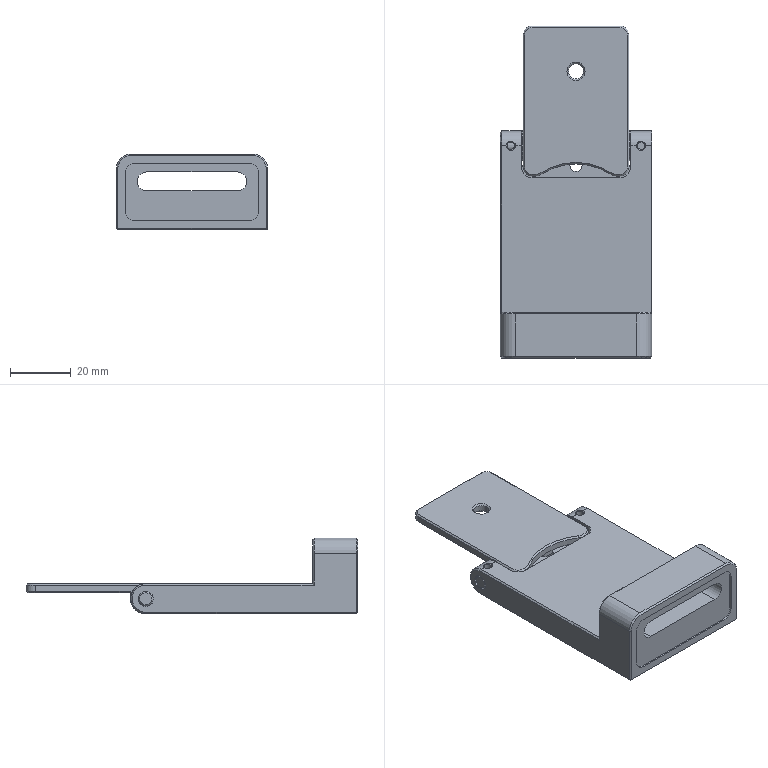Part | SolidWorks | 5 solids | 203 faces | box 50 x 109.5 x 25 mm | volume 40151 mm3 | plane 73 | cone 68 | cylinder 62 | commonest cylinder face diameters 6 x14 5 x12 10 x10 4 x7 2.5 x6 7 x4